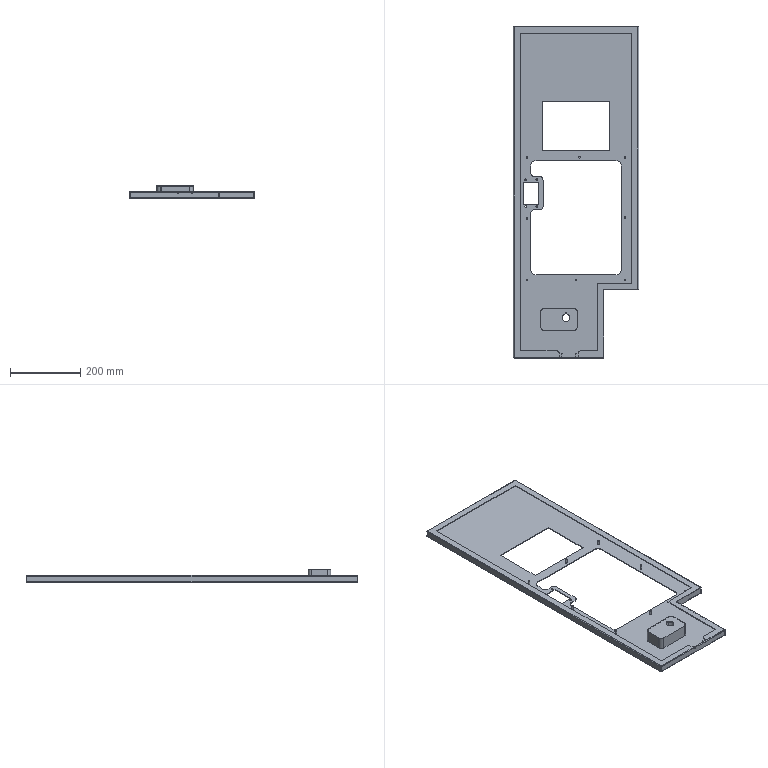Part | STEP file | 11-FG-JX01711 | 1 solid | 138 faces | box 358 x 948 x 37 mm | volume 620154 mm3 | plane 68 | cylinder 64 | sphere 6 | commonest cylinder face diameters 5 x16 20 x12 4 x11 5.5 x8 2.5 x4 3 x4